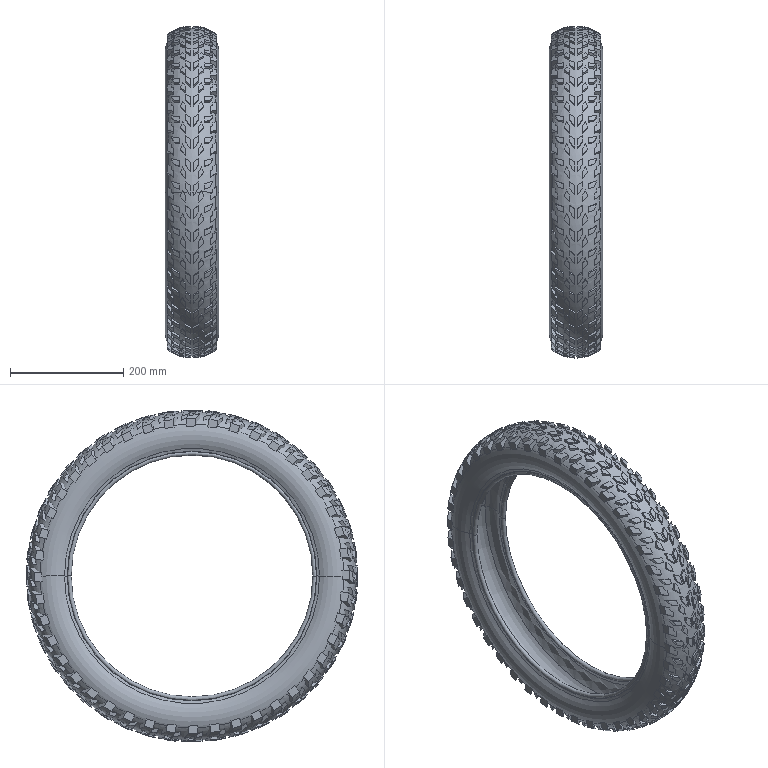Part | STEP file | BREP_89 | 1 solid | 1968 faces | box 94.52 x 587.169 x 587.169 mm | volume 1952183 mm3 | plane 1584 | torus 360 | other 24